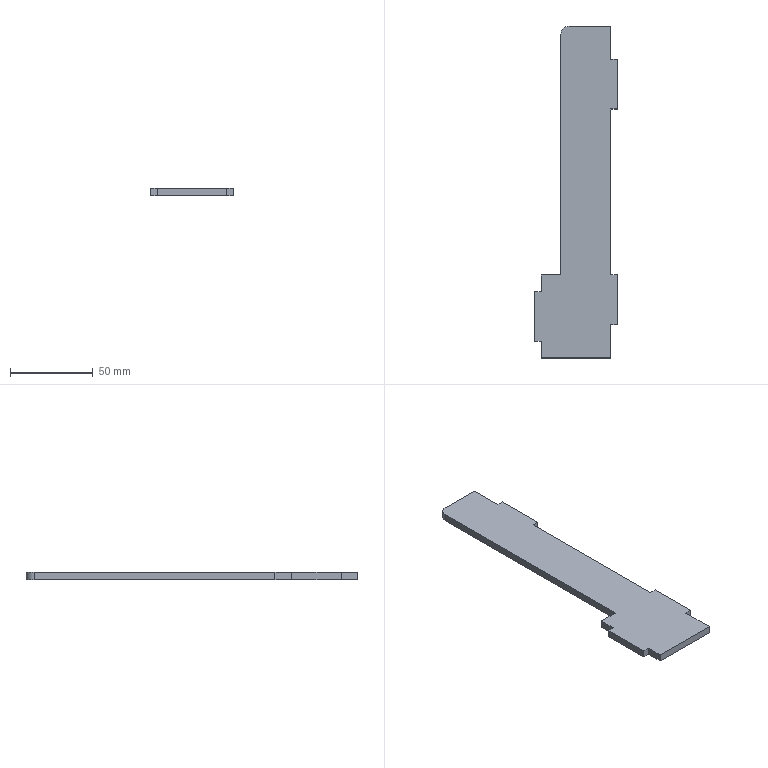Part | SolidWorks | features FlatPattern 1, SMBaseFlange 1, SheetMetal 1 | 1 solid | 21 faces | box 49.8 x 200 x 4.5 mm | volume 31251 mm3 | plane 20 | cylinder 1 | commonest cylinder face diameters 10 x1
STEP:
#1=CARTESIAN_POINT('',(-1112.571,288.492,0.));
#2=VERTEX_POINT('',#1);
#3=CARTESIAN_POINT('',(-1112.571,308.492,0.));
#4=VERTEX_POINT('',#3);
#5=CARTESIAN_POINT('',(-1112.571,288.492,0.));
#6=DIRECTION('',(0.,1.,0.));
#7=VECTOR('',#6,1000.);
#8=LINE('',#5,#7);
#9=EDGE_CURVE('',#2,#4,#8,.T.);
#10=ORIENTED_EDGE('',*,*,#9,.F.);
#11=CARTESIAN_POINT('',(-1112.571,288.492,-4.5));
#12=VERTEX_POINT('',#11);
#13=CARTESIAN_POINT('',(-1112.571,288.492,-4.5));
#14=DIRECTION('',(0.,0.,1.));
#15=VECTOR('',#14,1000.);
#16=LINE('',#13,#15);
#17=EDGE_CURVE('',#12,#2,#16,.T.);
#18=ORIENTED_EDGE('',*,*,#17,.F.);
#19=CARTESIAN_POINT('',(-1112.571,308.492,-4.5));
#20=VERTEX_POINT('',#19);
#21=CARTESIAN_POINT('',(-1112.571,288.492,-4.5));
#22=DIRECTION('',(0.,1.,0.));
#23=VECTOR('',#22,1000.);
#24=LINE('',#21,#23);
#25=EDGE_CURVE('',#12,#20,#24,.T.);
#26=ORIENTED_EDGE('',*,*,#25,.T.);
#27=CARTESIAN_POINT('',(-1112.571,308.492,-4.5));
#28=DIRECTION('',(0.,0.,1.));
#29=VECTOR('',#28,1000.);
#30=LINE('',#27,#29);
#31=EDGE_CURVE('',#20,#4,#30,.T.);
#32=ORIENTED_EDGE('',*,*,#31,.T.);
#33=EDGE_LOOP('',(#10,#18,#26,#32));
#34=FACE_OUTER_BOUND('',#33,.T.);
#35=CARTESIAN_POINT('',(-1112.571,288.492,-4.5));
#36=DIRECTION('',(1.,0.,0.));
#37=DIRECTION('',(0.,0.,-1.));
#38=AXIS2_PLACEMENT_3D('',#35,#36,#37);
#39=PLANE('',#38);
#40=ADVANCED_FACE('',(#34),#39,.T.);
#41=CARTESIAN_POINT('',(-1108.571,288.492,0.));
#42=VERTEX_POINT('',#41);
#43=CARTESIAN_POINT('',(-1108.571,288.492,0.));
#44=DIRECTION('',(-1.,0.,0.));
#45=VECTOR('',#44,1000.);
#46=LINE('',#43,#45);
#47=EDGE_CURVE('',#42,#2,#46,.T.);
#48=ORIENTED_EDGE('',*,*,#47,.F.);
#49=CARTESIAN_POINT('',(-1108.571,288.492,-4.5));
#50=VERTEX_POINT('',#49);
#51=CARTESIAN_POINT('',(-1108.571,288.492,-4.5));
#52=DIRECTION('',(0.,0.,1.));
#53=VECTOR('',#52,1000.);
#54=LINE('',#51,#53);
#55=EDGE_CURVE('',#50,#42,#54,.T.);
#56=ORIENTED_EDGE('',*,*,#55,.F.);
#57=CARTESIAN_POINT('',(-1108.571,288.492,-4.5));
#58=DIRECTION('',(-1.,0.,0.));
#59=VECTOR('',#58,1000.);
#60=LINE('',#57,#59);
#61=EDGE_CURVE('',#50,#12,#60,.T.);
#62=ORIENTED_EDGE('',*,*,#61,.T.);
#63=ORIENTED_EDGE('',*,*,#17,.T.);
#64=EDGE_LOOP('',(#48,#56,#62,#63));
#65=FACE_OUTER_BOUND('',#64,.T.);
#66=CARTESIAN_POINT('',(-1108.571,288.492,-4.5));
#67=DIRECTION('',(0.,1.,0.));
#68=DIRECTION('',(0.,0.,1.));
#69=AXIS2_PLACEMENT_3D('',#66,#67,#68);
#70=PLANE('',#69);
#71=ADVANCED_FACE('',(#65),#70,.T.);
#72=CARTESIAN_POINT('',(-1108.571,258.492,0.));
#73=VERTEX_POINT('',#72);
#74=CARTESIAN_POINT('',(-1108.571,258.492,0.));
#75=DIRECTION('',(0.,1.,0.));
#76=VECTOR('',#75,1000.);
#77=LINE('',#74,#76);
#78=EDGE_CURVE('',#73,#42,#77,.T.);
#79=ORIENTED_EDGE('',*,*,#78,.F.);
#80=CARTESIAN_POINT('',(-1108.571,258.492,-4.5));
#81=VERTEX_POINT('',#80);
#82=CARTESIAN_POINT('',(-1108.571,258.492,-4.5));
#83=DIRECTION('',(0.,0.,1.));
#84=VECTOR('',#83,1000.);
#85=LINE('',#82,#84);
#86=EDGE_CURVE('',#81,#73,#85,.T.);
#87=ORIENTED_EDGE('',*,*,#86,.F.);
#88=CARTESIAN_POINT('',(-1108.571,258.492,-4.5));
#89=DIRECTION('',(0.,1.,0.));
#90=VECTOR('',#89,1000.);
#91=LINE('',#88,#90);
#92=EDGE_CURVE('',#81,#50,#91,.T.);
#93=ORIENTED_EDGE('',*,*,#92,.T.);
#94=ORIENTED_EDGE('',*,*,#55,.T.);
#95=EDGE_LOOP('',(#79,#87,#93,#94));
#96=FACE_OUTER_BOUND('',#95,.T.);
#97=CARTESIAN_POINT('',(-1108.571,258.492,-4.5));
#98=DIRECTION('',(1.,0.,0.));
#99=DIRECTION('',(0.,0.,-1.));
#100=AXIS2_PLACEMENT_3D('',#97,#98,#99);
#101=PLANE('',#100);
#102=ADVANCED_FACE('',(#96),#101,.T.);
#103=CARTESIAN_POINT('',(-1112.571,258.492,0.));
#104=VERTEX_POINT('',#103);
#105=CARTESIAN_POINT('',(-1112.571,258.492,0.));
#106=DIRECTION('',(1.,0.,0.));
#107=VECTOR('',#106,1000.);
#108=LINE('',#105,#107);
#109=EDGE_CURVE('',#104,#73,#108,.T.);
#110=ORIENTED_EDGE('',*,*,#109,.F.);
#111=CARTESIAN_POINT('',(-1112.571,258.492,-4.5));
#112=VERTEX_POINT('',#111);
#113=CARTESIAN_POINT('',(-1112.571,258.492,-4.5));
#114=DIRECTION('',(0.,0.,1.));
#115=VECTOR('',#114,1000.);
#116=LINE('',#113,#115);
#117=EDGE_CURVE('',#112,#104,#116,.T.);
#118=ORIENTED_EDGE('',*,*,#117,.F.);
#119=CARTESIAN_POINT('',(-1112.571,258.492,-4.5));
#120=DIRECTION('',(1.,0.,0.));
#121=VECTOR('',#120,1000.);
#122=LINE('',#119,#121);
#123=EDGE_CURVE('',#112,#81,#122,.T.);
#124=ORIENTED_EDGE('',*,*,#123,.T.);
#125=ORIENTED_EDGE('',*,*,#86,.T.);
#126=EDGE_LOOP('',(#110,#118,#124,#125));
#127=FACE_OUTER_BOUND('',#126,.T.);
#128=CARTESIAN_POINT('',(-1112.571,258.492,-4.5));
#129=DIRECTION('',(0.,-1.,0.));
#130=DIRECTION('',(0.,0.,-1.));
#131=AXIS2_PLACEMENT_3D('',#128,#129,#130);
#132=PLANE('',#131);
#133=ADVANCED_FACE('',(#127),#132,.T.);
#134=CARTESIAN_POINT('',(-1112.571,158.492,0.));
#135=VERTEX_POINT('',#134);
#136=CARTESIAN_POINT('',(-1112.571,158.492,0.));
#137=DIRECTION('',(0.,1.,0.));
#138=VECTOR('',#137,1000.);
#139=LINE('',#136,#138);
#140=EDGE_CURVE('',#135,#104,#139,.T.);
#141=ORIENTED_EDGE('',*,*,#140,.F.);
#142=CARTESIAN_POINT('',(-1112.571,158.492,-4.5));
#143=VERTEX_POINT('',#142);
#144=CARTESIAN_POINT('',(-1112.571,158.492,-4.5));
#145=DIRECTION('',(0.,0.,1.));
#146=VECTOR('',#145,1000.);
#147=LINE('',#144,#146);
#148=EDGE_CURVE('',#143,#135,#147,.T.);
#149=ORIENTED_EDGE('',*,*,#148,.F.);
#150=CARTESIAN_POINT('',(-1112.571,158.492,-4.5));
#151=DIRECTION('',(0.,1.,0.));
#152=VECTOR('',#151,1000.);
#153=LINE('',#150,#152);
#154=EDGE_CURVE('',#143,#112,#153,.T.);
#155=ORIENTED_EDGE('',*,*,#154,.T.);
#156=ORIENTED_EDGE('',*,*,#117,.T.);
#157=EDGE_LOOP('',(#141,#149,#155,#156));
#158=FACE_OUTER_BOUND('',#157,.T.);
#159=CARTESIAN_POINT('',(-1112.571,158.492,-4.5));
#160=DIRECTION('',(1.,0.,0.));
#161=DIRECTION('',(0.,0.,-1.));
#162=AXIS2_PLACEMENT_3D('',#159,#160,#161);
#163=PLANE('',#162);
#164=ADVANCED_FACE('',(#158),#163,.T.);
#165=CARTESIAN_POINT('',(-1108.571,158.492,0.));
#166=VERTEX_POINT('',#165);
#167=CARTESIAN_POINT('',(-1108.571,158.492,0.));
#168=DIRECTION('',(-1.,0.,0.));
#169=VECTOR('',#168,1000.);
#170=LINE('',#167,#169);
#171=EDGE_CURVE('',#166,#135,#170,.T.);
#172=ORIENTED_EDGE('',*,*,#171,.F.);
#173=CARTESIAN_POINT('',(-1108.571,158.492,-4.5));
#174=VERTEX_POINT('',#173);
#175=CARTESIAN_POINT('',(-1108.571,158.492,-4.5));
#176=DIRECTION('',(0.,0.,1.));
#177=VECTOR('',#176,1000.);
#178=LINE('',#175,#177);
#179=EDGE_CURVE('',#174,#166,#178,.T.);
#180=ORIENTED_EDGE('',*,*,#179,.F.);
#181=CARTESIAN_POINT('',(-1108.571,158.492,-4.5));
#182=DIRECTION('',(-1.,0.,0.));
#183=VECTOR('',#182,1000.);
#184=LINE('',#181,#183);
#185=EDGE_CURVE('',#174,#143,#184,.T.);
#186=ORIENTED_EDGE('',*,*,#185,.T.);
#187=ORIENTED_EDGE('',*,*,#148,.T.);
#188=EDGE_LOOP('',(#172,#180,#186,#187));
#189=FACE_OUTER_BOUND('',#188,.T.);
#190=CARTESIAN_POINT('',(-1108.571,158.492,-4.5));
#191=DIRECTION('',(0.,1.,0.));
#192=DIRECTION('',(0.,0.,1.));
#193=AXIS2_PLACEMENT_3D('',#190,#191,#192);
#194=PLANE('',#193);
#195=ADVANCED_FACE('',(#189),#194,.T.);
#196=CARTESIAN_POINT('',(-1108.571,128.492,0.));
#197=VERTEX_POINT('',#196);
#198=CARTESIAN_POINT('',(-1108.571,128.492,0.));
#199=DIRECTION('',(0.,1.,0.));
#200=VECTOR('',#199,1000.);
#201=LINE('',#198,#200);
#202=EDGE_CURVE('',#197,#166,#201,.T.);
#203=ORIENTED_EDGE('',*,*,#202,.F.);
#204=CARTESIAN_POINT('',(-1108.571,128.492,-4.5));
#205=VERTEX_POINT('',#204);
#206=CARTESIAN_POINT('',(-1108.571,128.492,-4.5));
#207=DIRECTION('',(0.,0.,1.));
#208=VECTOR('',#207,1000.);
#209=LINE('',#206,#208);
#210=EDGE_CURVE('',#205,#197,#209,.T.);
#211=ORIENTED_EDGE('',*,*,#210,.F.);
#212=CARTESIAN_POINT('',(-1108.571,128.492,-4.5));
#213=DIRECTION('',(0.,1.,0.));
#214=VECTOR('',#213,1000.);
#215=LINE('',#212,#214);
#216=EDGE_CURVE('',#205,#174,#215,.T.);
#217=ORIENTED_EDGE('',*,*,#216,.T.);
#218=ORIENTED_EDGE('',*,*,#179,.T.);
#219=EDGE_LOOP('',(#203,#211,#217,#218));
#220=FACE_OUTER_BOUND('',#219,.T.);
#221=CARTESIAN_POINT('',(-1108.571,128.492,-4.5));
#222=DIRECTION('',(1.,0.,0.));
#223=DIRECTION('',(0.,0.,-1.));
#224=AXIS2_PLACEMENT_3D('',#221,#222,#223);
#225=PLANE('',#224);
#226=ADVANCED_FACE('',(#220),#225,.T.);
#227=CARTESIAN_POINT('',(-1112.571,128.492,0.));
#228=VERTEX_POINT('',#227);
#229=CARTESIAN_POINT('',(-1112.571,128.492,0.));
#230=DIRECTION('',(1.,0.,0.));
#231=VECTOR('',#230,1000.);
#232=LINE('',#229,#231);
#233=EDGE_CURVE('',#228,#197,#232,.T.);
#234=ORIENTED_EDGE('',*,*,#233,.F.);
#235=CARTESIAN_POINT('',(-1112.571,128.492,-4.5));
#236=VERTEX_POINT('',#235);
#237=CARTESIAN_POINT('',(-1112.571,128.492,-4.5));
#238=DIRECTION('',(0.,0.,1.));
#239=VECTOR('',#238,1000.);
#240=LINE('',#237,#239);
#241=EDGE_CURVE('',#236,#228,#240,.T.);
#242=ORIENTED_EDGE('',*,*,#241,.F.);
#243=CARTESIAN_POINT('',(-1112.571,128.492,-4.5));
#244=DIRECTION('',(1.,0.,0.));
#245=VECTOR('',#244,1000.);
#246=LINE('',#243,#245);
#247=EDGE_CURVE('',#236,#205,#246,.T.);
#248=ORIENTED_EDGE('',*,*,#247,.T.);
#249=ORIENTED_EDGE('',*,*,#210,.T.);
#250=EDGE_LOOP('',(#234,#242,#248,#249));
#251=FACE_OUTER_BOUND('',#250,.T.);
#252=CARTESIAN_POINT('',(-1112.571,128.492,-4.5));
#253=DIRECTION('',(0.,-1.,0.));
#254=DIRECTION('',(0.,0.,-1.));
#255=AXIS2_PLACEMENT_3D('',#252,#253,#254);
#256=PLANE('',#255);
#257=ADVANCED_FACE('',(#251),#256,.T.);
#258=CARTESIAN_POINT('',(-1112.571,108.492,0.));
#259=VERTEX_POINT('',#258);
#260=CARTESIAN_POINT('',(-1112.571,108.492,0.));
#261=DIRECTION('',(0.,1.,0.));
#262=VECTOR('',#261,1000.);
#263=LINE('',#260,#262);
#264=EDGE_CURVE('',#259,#228,#263,.T.);
#265=ORIENTED_EDGE('',*,*,#264,.F.);
#266=CARTESIAN_POINT('',(-1112.571,108.492,-4.5));
#267=VERTEX_POINT('',#266);
#268=CARTESIAN_POINT('',(-1112.571,108.492,-4.5));
#269=DIRECTION('',(0.,0.,1.));
#270=VECTOR('',#269,1000.);
#271=LINE('',#268,#270);
#272=EDGE_CURVE('',#267,#259,#271,.T.);
#273=ORIENTED_EDGE('',*,*,#272,.F.);
#274=CARTESIAN_POINT('',(-1112.571,108.492,-4.5));
#275=DIRECTION('',(0.,1.,0.));
#276=VECTOR('',#275,1000.);
#277=LINE('',#274,#276);
#278=EDGE_CURVE('',#267,#236,#277,.T.);
#279=ORIENTED_EDGE('',*,*,#278,.T.);
#280=ORIENTED_EDGE('',*,*,#241,.T.);
#281=EDGE_LOOP('',(#265,#273,#279,#280));
#282=FACE_OUTER_BOUND('',#281,.T.);
#283=CARTESIAN_POINT('',(-1112.571,108.492,-4.5));
#284=DIRECTION('',(1.,0.,0.));
#285=DIRECTION('',(0.,0.,-1.));
#286=AXIS2_PLACEMENT_3D('',#283,#284,#285);
#287=PLANE('',#286);
#288=ADVANCED_FACE('',(#282),#287,.T.);
#289=CARTESIAN_POINT('',(-1154.371,108.492,0.));
#290=VERTEX_POINT('',#289);
#291=CARTESIAN_POINT('',(-1154.371,108.492,0.));
#292=DIRECTION('',(1.,0.,0.));
#293=VECTOR('',#292,1000.);
#294=LINE('',#291,#293);
#295=EDGE_CURVE('',#290,#259,#294,.T.);
#296=ORIENTED_EDGE('',*,*,#295,.F.);
#297=CARTESIAN_POINT('',(-1154.371,108.492,-4.5));
#298=VERTEX_POINT('',#297);
#299=CARTESIAN_POINT('',(-1154.371,108.492,-4.5));
#300=DIRECTION('',(0.,0.,1.));
#301=VECTOR('',#300,1000.);
#302=LINE('',#299,#301);
#303=EDGE_CURVE('',#298,#290,#302,.T.);
#304=ORIENTED_EDGE('',*,*,#303,.F.);
#305=CARTESIAN_POINT('',(-1154.371,108.492,-4.5));
#306=DIRECTION('',(1.,0.,0.));
#307=VECTOR('',#306,1000.);
#308=LINE('',#305,#307);
#309=EDGE_CURVE('',#298,#267,#308,.T.);
#310=ORIENTED_EDGE('',*,*,#309,.T.);
#311=ORIENTED_EDGE('',*,*,#272,.T.);
#312=EDGE_LOOP('',(#296,#304,#310,#311));
#313=FACE_OUTER_BOUND('',#312,.T.);
#314=CARTESIAN_POINT('',(-1154.371,108.492,-4.5));
#315=DIRECTION('',(0.,-1.,0.));
#316=DIRECTION('',(0.,0.,-1.));
#317=AXIS2_PLACEMENT_3D('',#314,#315,#316);
#318=PLANE('',#317);
#319=ADVANCED_FACE('',(#313),#318,.T.);
#320=CARTESIAN_POINT('',(-1154.371,118.492,0.));
#321=VERTEX_POINT('',#320);
#322=CARTESIAN_POINT('',(-1154.371,118.492,0.));
#323=DIRECTION('',(0.,-1.,0.));
#324=VECTOR('',#323,1000.);
#325=LINE('',#322,#324);
#326=EDGE_CURVE('',#321,#290,#325,.T.);
#327=ORIENTED_EDGE('',*,*,#326,.F.);
#328=CARTESIAN_POINT('',(-1154.371,118.492,-4.5));
#329=VERTEX_POINT('',#328);
#330=CARTESIAN_POINT('',(-1154.371,118.492,-4.5));
#331=DIRECTION('',(0.,0.,1.));
#332=VECTOR('',#331,1000.);
#333=LINE('',#330,#332);
#334=EDGE_CURVE('',#329,#321,#333,.T.);
#335=ORIENTED_EDGE('',*,*,#334,.F.);
#336=CARTESIAN_POINT('',(-1154.371,118.492,-4.5));
#337=DIRECTION('',(0.,-1.,0.));
#338=VECTOR('',#337,1000.);
#339=LINE('',#336,#338);
#340=EDGE_CURVE('',#329,#298,#339,.T.);
#341=ORIENTED_EDGE('',*,*,#340,.T.);
#342=ORIENTED_EDGE('',*,*,#303,.T.);
#343=EDGE_LOOP('',(#327,#335,#341,#342));
#344=FACE_OUTER_BOUND('',#343,.T.);
#345=CARTESIAN_POINT('',(-1154.371,118.492,-4.5));
#346=DIRECTION('',(-1.,0.,0.));
#347=DIRECTION('',(0.,0.,1.));
#348=AXIS2_PLACEMENT_3D('',#345,#346,#347);
#349=PLANE('',#348);
#350=ADVANCED_FACE('',(#344),#349,.T.);
#351=CARTESIAN_POINT('',(-1158.371,118.492,0.));
#352=VERTEX_POINT('',#351);
#353=CARTESIAN_POINT('',(-1154.371,118.492,0.));
#354=DIRECTION('',(1.,0.,0.));
#355=VECTOR('',#354,1000.);
#356=LINE('',#353,#355);
#357=EDGE_CURVE('',#352,#321,#356,.T.);
#358=ORIENTED_EDGE('',*,*,#357,.F.);
#359=CARTESIAN_POINT('',(-1158.371,118.492,-4.5));
#360=VERTEX_POINT('',#359);
#361=CARTESIAN_POINT('',(-1158.371,118.492,-4.5));
#362=DIRECTION('',(0.,0.,1.));
#363=VECTOR('',#362,1000.);
#364=LINE('',#361,#363);
#365=EDGE_CURVE('',#360,#352,#364,.T.);
#366=ORIENTED_EDGE('',*,*,#365,.F.);
#367=CARTESIAN_POINT('',(-1154.371,118.492,-4.5));
#368=DIRECTION('',(1.,0.,0.));
#369=VECTOR('',#368,1000.);
#370=LINE('',#367,#369);
#371=EDGE_CURVE('',#360,#329,#370,.T.);
#372=ORIENTED_EDGE('',*,*,#371,.T.);
#373=ORIENTED_EDGE('',*,*,#334,.T.);
#374=EDGE_LOOP('',(#358,#366,#372,#373));
#375=FACE_OUTER_BOUND('',#374,.T.);
#376=CARTESIAN_POINT('',(-1154.371,118.492,-4.5));
#377=DIRECTION('',(0.,-1.,0.));
#378=DIRECTION('',(0.,0.,-1.));
#379=AXIS2_PLACEMENT_3D('',#376,#377,#378);
#380=PLANE('',#379);
#381=ADVANCED_FACE('',(#375),#380,.T.);
#382=CARTESIAN_POINT('',(-1158.371,148.492,0.));
#383=VERTEX_POINT('',#382);
#384=CARTESIAN_POINT('',(-1158.371,118.492,0.));
#385=DIRECTION('',(0.,-1.,0.));
#386=VECTOR('',#385,1000.);
#387=LINE('',#384,#386);
#388=EDGE_CURVE('',#383,#352,#387,.T.);
#389=ORIENTED_EDGE('',*,*,#388,.F.);
#390=CARTESIAN_POINT('',(-1158.371,148.492,-4.5));
#391=VERTEX_POINT('',#390);
#392=CARTESIAN_POINT('',(-1158.371,148.492,-4.5));
#393=DIRECTION('',(0.,0.,1.));
#394=VECTOR('',#393,1000.);
#395=LINE('',#392,#394);
#396=EDGE_CURVE('',#391,#383,#395,.T.);
#397=ORIENTED_EDGE('',*,*,#396,.F.);
#398=CARTESIAN_POINT('',(-1158.371,118.492,-4.5));
#399=DIRECTION('',(0.,-1.,0.));
#400=VECTOR('',#399,1000.);
#401=LINE('',#398,#400);
#402=EDGE_CURVE('',#391,#360,#401,.T.);
#403=ORIENTED_EDGE('',*,*,#402,.T.);
#404=ORIENTED_EDGE('',*,*,#365,.T.);
#405=EDGE_LOOP('',(#389,#397,#403,#404));
#406=FACE_OUTER_BOUND('',#405,.T.);
#407=CARTESIAN_POINT('',(-1158.371,118.492,-4.5));
#408=DIRECTION('',(-1.,0.,0.));
#409=DIRECTION('',(0.,0.,1.));
#410=AXIS2_PLACEMENT_3D('',#407,#408,#409);
#411=PLANE('',#410);
#412=ADVANCED_FACE('',(#406),#411,.T.);
#413=CARTESIAN_POINT('',(-1154.371,148.492,0.));
#414=VERTEX_POINT('',#413);
#415=CARTESIAN_POINT('',(-1158.371,148.492,0.));
#416=DIRECTION('',(-1.,0.,0.));
#417=VECTOR('',#416,1000.);
#418=LINE('',#415,#417);
#419=EDGE_CURVE('',#414,#383,#418,.T.);
#420=ORIENTED_EDGE('',*,*,#419,.F.);
#421=CARTESIAN_POINT('',(-1154.371,148.492,-4.5));
#422=VERTEX_POINT('',#421);
#423=CARTESIAN_POINT('',(-1154.371,148.492,-4.5));
#424=DIRECTION('',(0.,0.,1.));
#425=VECTOR('',#424,1000.);
#426=LINE('',#423,#425);
#427=EDGE_CURVE('',#422,#414,#426,.T.);
#428=ORIENTED_EDGE('',*,*,#427,.F.);
#429=CARTESIAN_POINT('',(-1158.371,148.492,-4.5));
#430=DIRECTION('',(-1.,0.,0.));
#431=VECTOR('',#430,1000.);
#432=LINE('',#429,#431);
#433=EDGE_CURVE('',#422,#391,#432,.T.);
#434=ORIENTED_EDGE('',*,*,#433,.T.);
#435=ORIENTED_EDGE('',*,*,#396,.T.);
#436=EDGE_LOOP('',(#420,#428,#434,#435));
#437=FACE_OUTER_BOUND('',#436,.T.);
#438=CARTESIAN_POINT('',(-1158.371,148.492,-4.5));
#439=DIRECTION('',(0.,1.,0.));
#440=DIRECTION('',(0.,0.,1.));
#441=AXIS2_PLACEMENT_3D('',#438,#439,#440);
#442=PLANE('',#441);
#443=ADVANCED_FACE('',(#437),#442,.T.);
#444=CARTESIAN_POINT('',(-1154.371,158.492,0.));
#445=VERTEX_POINT('',#444);
#446=CARTESIAN_POINT('',(-1154.371,158.492,0.));
#447=DIRECTION('',(0.,-1.,0.));
#448=VECTOR('',#447,1000.);
#449=LINE('',#446,#448);
#450=EDGE_CURVE('',#445,#414,#449,.T.);
#451=ORIENTED_EDGE('',*,*,#450,.F.);
#452=CARTESIAN_POINT('',(-1154.371,158.492,-4.5));
#453=VERTEX_POINT('',#452);
#454=CARTESIAN_POINT('',(-1154.371,158.492,-4.5));
#455=DIRECTION('',(0.,0.,1.));
#456=VECTOR('',#455,1000.);
#457=LINE('',#454,#456);
#458=EDGE_CURVE('',#453,#445,#457,.T.);
#459=ORIENTED_EDGE('',*,*,#458,.F.);
#460=CARTESIAN_POINT('',(-1154.371,158.492,-4.5));
#461=DIRECTION('',(0.,-1.,0.));
#462=VECTOR('',#461,1000.);
#463=LINE('',#460,#462);
#464=EDGE_CURVE('',#453,#422,#463,.T.);
#465=ORIENTED_EDGE('',*,*,#464,.T.);
#466=ORIENTED_EDGE('',*,*,#427,.T.);
#467=EDGE_LOOP('',(#451,#459,#465,#466));
#468=FACE_OUTER_BOUND('',#467,.T.);
#469=CARTESIAN_POINT('',(-1154.371,158.492,-4.5));
#470=DIRECTION('',(-1.,0.,0.));
#471=DIRECTION('',(0.,0.,1.));
#472=AXIS2_PLACEMENT_3D('',#469,#470,#471);
#473=PLANE('',#472);
#474=ADVANCED_FACE('',(#468),#473,.T.);
#475=CARTESIAN_POINT('',(-1142.571,158.492,0.));
#476=VERTEX_POINT('',#475);
#477=CARTESIAN_POINT('',(-1142.571,158.492,0.));
#478=DIRECTION('',(-1.,0.,0.));
#479=VECTOR('',#478,1000.);
#480=LINE('',#477,#479);
#481=EDGE_CURVE('',#476,#445,#480,.T.);
#482=ORIENTED_EDGE('',*,*,#481,.F.);
#483=CARTESIAN_POINT('',(-1142.571,158.492,-4.5));
#484=VERTEX_POINT('',#483);
#485=CARTESIAN_POINT('',(-1142.571,158.492,-4.5));
#486=DIRECTION('',(0.,0.,1.));
#487=VECTOR('',#486,1000.);
#488=LINE('',#485,#487);
#489=EDGE_CURVE('',#484,#476,#488,.T.);
#490=ORIENTED_EDGE('',*,*,#489,.F.);
#491=CARTESIAN_POINT('',(-1142.571,158.492,-4.5));
#492=DIRECTION('',(-1.,0.,0.));
#493=VECTOR('',#492,1000.);
#494=LINE('',#491,#493);
#495=EDGE_CURVE('',#484,#453,#494,.T.);
#496=ORIENTED_EDGE('',*,*,#495,.T.);
#497=ORIENTED_EDGE('',*,*,#458,.T.);
#498=EDGE_LOOP('',(#482,#490,#496,#497));
#499=FACE_OUTER_BOUND('',#498,.T.);
#500=CARTESIAN_POINT('',(-1142.571,158.492,-4.5));
#501=DIRECTION('',(0.,1.,0.));
#502=DIRECTION('',(0.,0.,1.));
#503=AXIS2_PLACEMENT_3D('',#500,#501,#502);
#504=PLANE('',#503);
#505=ADVANCED_FACE('',(#499),#504,.T.);
#506=CARTESIAN_POINT('',(-1142.571,303.492,0.));
#507=VERTEX_POINT('',#506);
#508=CARTESIAN_POINT('',(-1142.571,303.492,0.));
#509=DIRECTION('',(0.,-1.,0.));
#510=VECTOR('',#509,1000.);
#511=LINE('',#508,#510);
#512=EDGE_CURVE('',#507,#476,#511,.T.);
#513=ORIENTED_EDGE('',*,*,#512,.F.);
#514=CARTESIAN_POINT('',(-1142.571,303.492,-4.5));
#515=VERTEX_POINT('',#514);
#516=CARTESIAN_POINT('',(-1142.571,303.492,-4.5));
#517=DIRECTION('',(0.,0.,1.));
#518=VECTOR('',#517,1000.);
#519=LINE('',#516,#518);
#520=EDGE_CURVE('',#515,#507,#519,.T.);
#521=ORIENTED_EDGE('',*,*,#520,.F.);
#522=CARTESIAN_POINT('',(-1142.571,303.492,-4.5));
#523=DIRECTION('',(0.,-1.,0.));
#524=VECTOR('',#523,1000.);
#525=LINE('',#522,#524);
#526=EDGE_CURVE('',#515,#484,#525,.T.);
#527=ORIENTED_EDGE('',*,*,#526,.T.);
#528=ORIENTED_EDGE('',*,*,#489,.T.);
#529=EDGE_LOOP('',(#513,#521,#527,#528));
#530=FACE_OUTER_BOUND('',#529,.T.);
#531=CARTESIAN_POINT('',(-1142.571,303.492,-4.5));
#532=DIRECTION('',(-1.,0.,0.));
#533=DIRECTION('',(0.,0.,1.));
#534=AXIS2_PLACEMENT_3D('',#531,#532,#533);
#535=PLANE('',#534);
#536=ADVANCED_FACE('',(#530),#535,.T.);
#537=CARTESIAN_POINT('',(-1137.571,308.492,0.));
#538=VERTEX_POINT('',#537);
#539=CARTESIAN_POINT('',(-1137.571,303.492,0.));
#540=DIRECTION('',(0.,0.,1.));
#541=DIRECTION('',(1.,0.,0.));
#542=AXIS2_PLACEMENT_3D('',#539,#540,#541);
#543=CIRCLE('',#542,5.);
#544=EDGE_CURVE('',#538,#507,#543,.T.);
#545=ORIENTED_EDGE('',*,*,#544,.F.);
#546=CARTESIAN_POINT('',(-1137.571,308.492,-4.5));
#547=VERTEX_POINT('',#546);
#548=CARTESIAN_POINT('',(-1137.571,308.492,-4.5));
#549=DIRECTION('',(0.,0.,1.));
#550=VECTOR('',#549,1000.);
#551=LINE('',#548,#550);
#552=EDGE_CURVE('',#547,#538,#551,.T.);
#553=ORIENTED_EDGE('',*,*,#552,.F.);
#554=CARTESIAN_POINT('',(-1137.571,303.492,-4.5));
#555=DIRECTION('',(0.,0.,1.));
#556=DIRECTION('',(1.,0.,0.));
#557=AXIS2_PLACEMENT_3D('',#554,#555,#556);
#558=CIRCLE('',#557,5.);
#559=EDGE_CURVE('',#547,#515,#558,.T.);
#560=ORIENTED_EDGE('',*,*,#559,.T.);
#561=ORIENTED_EDGE('',*,*,#520,.T.);
#562=EDGE_LOOP('',(#545,#553,#560,#561));
#563=FACE_OUTER_BOUND('',#562,.T.);
#564=CARTESIAN_POINT('',(-1137.571,303.492,-4.5));
#565=DIRECTION('',(0.,0.,1.));
#566=DIRECTION('',(1.,0.,0.));
#567=AXIS2_PLACEMENT_3D('',#564,#565,#566);
#568=CYLINDRICAL_SURFACE('',#567,5.);
#569=ADVANCED_FACE('',(#563),#568,.T.);
#570=CARTESIAN_POINT('',(-1112.571,308.492,0.));
#571=DIRECTION('',(-1.,0.,0.));
#572=VECTOR('',#571,1000.);
#573=LINE('',#570,#572);
#574=EDGE_CURVE('',#4,#538,#573,.T.);
#575=ORIENTED_EDGE('',*,*,#574,.F.);
#576=ORIENTED_EDGE('',*,*,#31,.F.);
#577=CARTESIAN_POINT('',(-1112.571,308.492,-4.5));
#578=DIRECTION('',(-1.,0.,0.));
#579=VECTOR('',#578,1000.);
#580=LINE('',#577,#579);
#581=EDGE_CURVE('',#20,#547,#580,.T.);
#582=ORIENTED_EDGE('',*,*,#581,.T.);
#583=ORIENTED_EDGE('',*,*,#552,.T.);
#584=EDGE_LOOP('',(#575,#576,#582,#583));
#585=FACE_OUTER_BOUND('',#584,.T.);
#586=CARTESIAN_POINT('',(-1112.571,308.492,-4.5));
#587=DIRECTION('',(0.,1.,0.));
#588=DIRECTION('',(0.,0.,1.));
#589=AXIS2_PLACEMENT_3D('',#586,#587,#588);
#590=PLANE('',#589);
#591=ADVANCED_FACE('',(#585),#590,.T.);
#592=ORIENTED_EDGE('',*,*,#25,.F.);
#593=ORIENTED_EDGE('',*,*,#61,.F.);
#594=ORIENTED_EDGE('',*,*,#92,.F.);
#595=ORIENTED_EDGE('',*,*,#123,.F.);
#596=ORIENTED_EDGE('',*,*,#154,.F.);
#597=ORIENTED_EDGE('',*,*,#185,.F.);
#598=ORIENTED_EDGE('',*,*,#216,.F.);
#599=ORIENTED_EDGE('',*,*,#247,.F.);
#600=ORIENTED_EDGE('',*,*,#278,.F.);
#601=ORIENTED_EDGE('',*,*,#309,.F.);
#602=ORIENTED_EDGE('',*,*,#340,.F.);
#603=ORIENTED_EDGE('',*,*,#371,.F.);
#604=ORIENTED_EDGE('',*,*,#402,.F.);
#605=ORIENTED_EDGE('',*,*,#433,.F.);
#606=ORIENTED_EDGE('',*,*,#464,.F.);
#607=ORIENTED_EDGE('',*,*,#495,.F.);
#608=ORIENTED_EDGE('',*,*,#526,.F.);
#609=ORIENTED_EDGE('',*,*,#559,.F.);
#610=ORIENTED_EDGE('',*,*,#581,.F.);
#611=EDGE_LOOP('',(#592,#593,#594,#595,#596,#597,#598,#599,#600,#601,#602,#603,#604,#605,#606,#607,#608,#609,#610));
#612=FACE_OUTER_BOUND('',#611,.T.);
#613=CARTESIAN_POINT('',(-1137.571,303.492,-4.5));
#614=DIRECTION('',(0.,0.,1.));
#615=DIRECTION('',(1.,0.,0.));
#616=AXIS2_PLACEMENT_3D('',#613,#614,#615);
#617=PLANE('',#616);
#618=ADVANCED_FACE('',(#612),#617,.F.);
#619=ORIENTED_EDGE('',*,*,#9,.T.);
#620=ORIENTED_EDGE('',*,*,#574,.T.);
#621=ORIENTED_EDGE('',*,*,#544,.T.);
#622=ORIENTED_EDGE('',*,*,#512,.T.);
#623=ORIENTED_EDGE('',*,*,#481,.T.);
#624=ORIENTED_EDGE('',*,*,#450,.T.);
#625=ORIENTED_EDGE('',*,*,#419,.T.);
#626=ORIENTED_EDGE('',*,*,#388,.T.);
#627=ORIENTED_EDGE('',*,*,#357,.T.);
#628=ORIENTED_EDGE('',*,*,#326,.T.);
#629=ORIENTED_EDGE('',*,*,#295,.T.);
#630=ORIENTED_EDGE('',*,*,#264,.T.);
#631=ORIENTED_EDGE('',*,*,#233,.T.);
#632=ORIENTED_EDGE('',*,*,#202,.T.);
#633=ORIENTED_EDGE('',*,*,#171,.T.);
#634=ORIENTED_EDGE('',*,*,#140,.T.);
#635=ORIENTED_EDGE('',*,*,#109,.T.);
#636=ORIENTED_EDGE('',*,*,#78,.T.);
#637=ORIENTED_EDGE('',*,*,#47,.T.);
#638=EDGE_LOOP('',(#619,#620,#621,#622,#623,#624,#625,#626,#627,#628,#629,#630,#631,#632,#633,#634,#635,#636,#637));
#639=FACE_OUTER_BOUND('',#638,.T.);
#640=CARTESIAN_POINT('',(-1137.571,303.492,0.));
#641=DIRECTION('',(0.,0.,1.));
#642=DIRECTION('',(1.,0.,0.));
#643=AXIS2_PLACEMENT_3D('',#640,#641,#642);
#644=PLANE('',#643);
#645=ADVANCED_FACE('',(#639),#644,.T.);
#646=CLOSED_SHELL('',(#40,#71,#102,#133,#164,#195,#226,#257,#288,#319,#350,#381,#412,#443,#474,#505,#536,#569,#591,#618,#645));
#647=MANIFOLD_SOLID_BREP('',#646);
#648=CARTESIAN_POINT('',(0.,0.,0.));
#649=DIRECTION('',(0.,0.,1.));
#650=DIRECTION('',(1.,0.,0.));
#651=AXIS2_PLACEMENT_3D('',#648,#649,#650);
#652=(LENGTH_UNIT()NAMED_UNIT(*)SI_UNIT(.MILLI.,.METRE.));
#653=UNCERTAINTY_MEASURE_WITH_UNIT(LENGTH_MEASURE(0.00001),#652,'','');
#654=(NAMED_UNIT(*)PLANE_ANGLE_UNIT()SI_UNIT($,.RADIAN.));
#655=(NAMED_UNIT(*)SI_UNIT($,.STERADIAN.)SOLID_ANGLE_UNIT());
#656=(GEOMETRIC_REPRESENTATION_CONTEXT(3)GLOBAL_UNCERTAINTY_ASSIGNED_CONTEXT((#653))GLOBAL_UNIT_ASSIGNED_CONTEXT((#652,#654,#655))REPRESENTATION_CONTEXT('',''));
#657=ADVANCED_BREP_SHAPE_REPRESENTATION('',(#647,#651),#656);